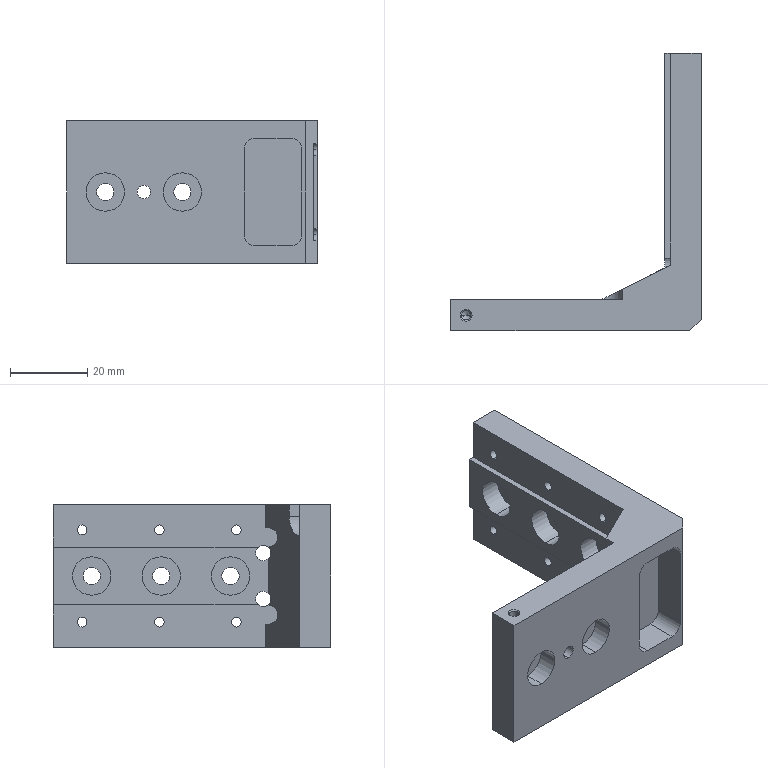Part | STEP file | 1 solid | 116 faces | box 65 x 72 x 37 mm | volume 34772 mm3 | cylinder 65 | plane 33 | cone 18 | commonest cylinder face diameters 2.5 x26 10 x11 4.5 x10 3 x4 4 x4 6 x4